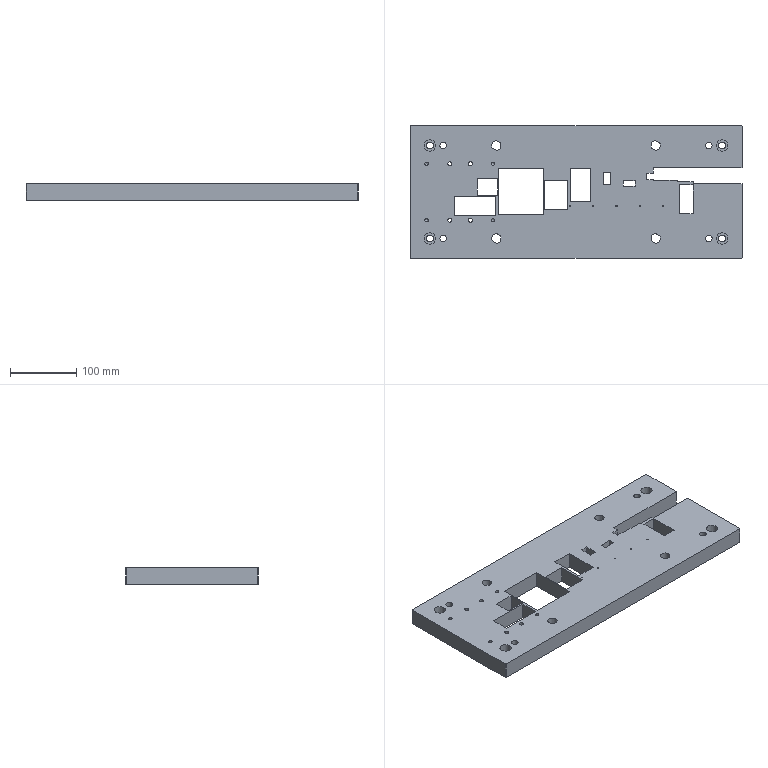Part | NX | features BREP 1 | 1 solid | 103 faces | box 500 x 200 x 25 mm | volume 2084515 mm3 | plane 66 | cylinder 33 | cone 4 | commonest cylinder face diameters 2 x5 5 x4 6 x4 10 x4 10.5 x4 14 x4